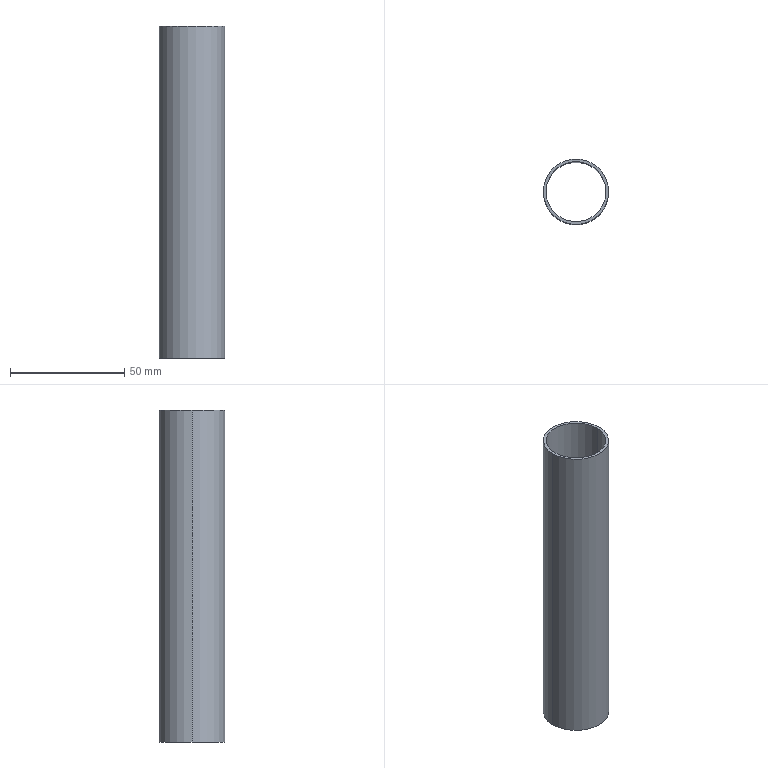Part | STEP file | 28._28.6X145 | 1 solid | 6 faces | box 28.6 x 28.6 x 145 mm | volume 14978 mm3 | cylinder 4 | plane 2 | commonest cylinder face diameters 26.2 x2 28.6 x2
STEP:
#1=CARTESIAN_POINT('',(13.1,0.,0.));
#2=VERTEX_POINT('',#1);
#3=CARTESIAN_POINT('',(-13.1,0.,0.));
#4=VERTEX_POINT('',#3);
#5=CARTESIAN_POINT('',(0.,0.,0.));
#6=DIRECTION('',(0.,0.,-1.));
#7=DIRECTION('',(1.,0.,0.));
#8=AXIS2_PLACEMENT_3D('',#5,#6,#7);
#9=CIRCLE('',#8,13.1);
#10=EDGE_CURVE('',#2,#4,#9,.T.);
#11=ORIENTED_EDGE('',*,*,#10,.T.);
#12=CARTESIAN_POINT('',(-13.1,0.,145.));
#13=VERTEX_POINT('',#12);
#14=CARTESIAN_POINT('',(-13.1,0.,0.));
#15=DIRECTION('',(0.,0.,1.));
#16=VECTOR('',#15,1000.);
#17=LINE('',#14,#16);
#18=EDGE_CURVE('',#4,#13,#17,.T.);
#19=ORIENTED_EDGE('',*,*,#18,.T.);
#20=CARTESIAN_POINT('',(13.1,0.,145.));
#21=VERTEX_POINT('',#20);
#22=CARTESIAN_POINT('',(0.,0.,145.));
#23=DIRECTION('',(0.,0.,-1.));
#24=DIRECTION('',(1.,0.,0.));
#25=AXIS2_PLACEMENT_3D('',#22,#23,#24);
#26=CIRCLE('',#25,13.1);
#27=EDGE_CURVE('',#21,#13,#26,.T.);
#28=ORIENTED_EDGE('',*,*,#27,.F.);
#29=CARTESIAN_POINT('',(13.1,0.,0.));
#30=DIRECTION('',(0.,0.,1.));
#31=VECTOR('',#30,1000.);
#32=LINE('',#29,#31);
#33=EDGE_CURVE('',#2,#21,#32,.T.);
#34=ORIENTED_EDGE('',*,*,#33,.F.);
#35=EDGE_LOOP('',(#11,#19,#28,#34));
#36=FACE_OUTER_BOUND('',#35,.T.);
#37=CARTESIAN_POINT('',(0.,0.,0.));
#38=DIRECTION('',(0.,0.,1.));
#39=DIRECTION('',(1.,0.,0.));
#40=AXIS2_PLACEMENT_3D('',#37,#38,#39);
#41=CYLINDRICAL_SURFACE('',#40,13.1);
#42=ADVANCED_FACE('',(#36),#41,.F.);
#43=CARTESIAN_POINT('',(14.3,0.,0.));
#44=VERTEX_POINT('',#43);
#45=CARTESIAN_POINT('',(-14.3,0.,0.));
#46=VERTEX_POINT('',#45);
#47=CARTESIAN_POINT('',(0.,0.,0.));
#48=DIRECTION('',(0.,0.,1.));
#49=DIRECTION('',(1.,0.,0.));
#50=AXIS2_PLACEMENT_3D('',#47,#48,#49);
#51=CIRCLE('',#50,14.3);
#52=EDGE_CURVE('',#44,#46,#51,.T.);
#53=ORIENTED_EDGE('',*,*,#52,.T.);
#54=CARTESIAN_POINT('',(-14.3,0.,145.));
#55=VERTEX_POINT('',#54);
#56=CARTESIAN_POINT('',(-14.3,0.,0.));
#57=DIRECTION('',(0.,0.,1.));
#58=VECTOR('',#57,1000.);
#59=LINE('',#56,#58);
#60=EDGE_CURVE('',#46,#55,#59,.T.);
#61=ORIENTED_EDGE('',*,*,#60,.T.);
#62=CARTESIAN_POINT('',(14.3,0.,145.));
#63=VERTEX_POINT('',#62);
#64=CARTESIAN_POINT('',(0.,0.,145.));
#65=DIRECTION('',(0.,0.,1.));
#66=DIRECTION('',(1.,0.,0.));
#67=AXIS2_PLACEMENT_3D('',#64,#65,#66);
#68=CIRCLE('',#67,14.3);
#69=EDGE_CURVE('',#63,#55,#68,.T.);
#70=ORIENTED_EDGE('',*,*,#69,.F.);
#71=CARTESIAN_POINT('',(14.3,0.,0.));
#72=DIRECTION('',(0.,0.,1.));
#73=VECTOR('',#72,1000.);
#74=LINE('',#71,#73);
#75=EDGE_CURVE('',#44,#63,#74,.T.);
#76=ORIENTED_EDGE('',*,*,#75,.F.);
#77=EDGE_LOOP('',(#53,#61,#70,#76));
#78=FACE_OUTER_BOUND('',#77,.T.);
#79=CARTESIAN_POINT('',(0.,0.,0.));
#80=DIRECTION('',(0.,0.,1.));
#81=DIRECTION('',(1.,0.,0.));
#82=AXIS2_PLACEMENT_3D('',#79,#80,#81);
#83=CYLINDRICAL_SURFACE('',#82,14.3);
#84=ADVANCED_FACE('',(#78),#83,.T.);
#85=ORIENTED_EDGE('',*,*,#10,.F.);
#86=CARTESIAN_POINT('',(0.,0.,0.));
#87=DIRECTION('',(0.,0.,-1.));
#88=DIRECTION('',(1.,0.,0.));
#89=AXIS2_PLACEMENT_3D('',#86,#87,#88);
#90=CIRCLE('',#89,13.1);
#91=EDGE_CURVE('',#4,#2,#90,.T.);
#92=ORIENTED_EDGE('',*,*,#91,.F.);
#93=EDGE_LOOP('',(#85,#92));
#94=FACE_BOUND('',#93,.T.);
#95=ORIENTED_EDGE('',*,*,#52,.F.);
#96=CARTESIAN_POINT('',(0.,0.,0.));
#97=DIRECTION('',(0.,0.,1.));
#98=DIRECTION('',(1.,0.,0.));
#99=AXIS2_PLACEMENT_3D('',#96,#97,#98);
#100=CIRCLE('',#99,14.3);
#101=EDGE_CURVE('',#46,#44,#100,.T.);
#102=ORIENTED_EDGE('',*,*,#101,.F.);
#103=EDGE_LOOP('',(#95,#102));
#104=FACE_OUTER_BOUND('',#103,.T.);
#105=CARTESIAN_POINT('',(0.,0.,0.));
#106=DIRECTION('',(0.,0.,1.));
#107=DIRECTION('',(1.,0.,0.));
#108=AXIS2_PLACEMENT_3D('',#105,#106,#107);
#109=PLANE('',#108);
#110=ADVANCED_FACE('',(#94,#104),#109,.F.);
#111=ORIENTED_EDGE('',*,*,#27,.T.);
#112=CARTESIAN_POINT('',(0.,0.,145.));
#113=DIRECTION('',(0.,0.,-1.));
#114=DIRECTION('',(1.,0.,0.));
#115=AXIS2_PLACEMENT_3D('',#112,#113,#114);
#116=CIRCLE('',#115,13.1);
#117=EDGE_CURVE('',#13,#21,#116,.T.);
#118=ORIENTED_EDGE('',*,*,#117,.T.);
#119=EDGE_LOOP('',(#111,#118));
#120=FACE_BOUND('',#119,.T.);
#121=ORIENTED_EDGE('',*,*,#69,.T.);
#122=CARTESIAN_POINT('',(0.,0.,145.));
#123=DIRECTION('',(0.,0.,1.));
#124=DIRECTION('',(1.,0.,0.));
#125=AXIS2_PLACEMENT_3D('',#122,#123,#124);
#126=CIRCLE('',#125,14.3);
#127=EDGE_CURVE('',#55,#63,#126,.T.);
#128=ORIENTED_EDGE('',*,*,#127,.T.);
#129=EDGE_LOOP('',(#121,#128));
#130=FACE_OUTER_BOUND('',#129,.T.);
#131=CARTESIAN_POINT('',(0.,0.,145.));
#132=DIRECTION('',(0.,0.,1.));
#133=DIRECTION('',(1.,0.,0.));
#134=AXIS2_PLACEMENT_3D('',#131,#132,#133);
#135=PLANE('',#134);
#136=ADVANCED_FACE('',(#120,#130),#135,.T.);
#137=ORIENTED_EDGE('',*,*,#60,.F.);
#138=ORIENTED_EDGE('',*,*,#101,.T.);
#139=ORIENTED_EDGE('',*,*,#75,.T.);
#140=ORIENTED_EDGE('',*,*,#127,.F.);
#141=EDGE_LOOP('',(#137,#138,#139,#140));
#142=FACE_OUTER_BOUND('',#141,.T.);
#143=CARTESIAN_POINT('',(0.,0.,0.));
#144=DIRECTION('',(0.,0.,1.));
#145=DIRECTION('',(1.,0.,0.));
#146=AXIS2_PLACEMENT_3D('',#143,#144,#145);
#147=CYLINDRICAL_SURFACE('',#146,14.3);
#148=ADVANCED_FACE('',(#142),#147,.T.);
#149=ORIENTED_EDGE('',*,*,#18,.F.);
#150=ORIENTED_EDGE('',*,*,#91,.T.);
#151=ORIENTED_EDGE('',*,*,#33,.T.);
#152=ORIENTED_EDGE('',*,*,#117,.F.);
#153=EDGE_LOOP('',(#149,#150,#151,#152));
#154=FACE_OUTER_BOUND('',#153,.T.);
#155=CARTESIAN_POINT('',(0.,0.,0.));
#156=DIRECTION('',(0.,0.,1.));
#157=DIRECTION('',(1.,0.,0.));
#158=AXIS2_PLACEMENT_3D('',#155,#156,#157);
#159=CYLINDRICAL_SURFACE('',#158,13.1);
#160=ADVANCED_FACE('',(#154),#159,.F.);
#161=CLOSED_SHELL('',(#42,#84,#110,#136,#148,#160));
#162=MANIFOLD_SOLID_BREP('',#161);
#163=CARTESIAN_POINT('',(0.,0.,0.));
#164=DIRECTION('',(0.,0.,1.));
#165=DIRECTION('',(1.,0.,0.));
#166=AXIS2_PLACEMENT_3D('',#163,#164,#165);
#167=(LENGTH_UNIT()NAMED_UNIT(*)SI_UNIT(.MILLI.,.METRE.));
#168=UNCERTAINTY_MEASURE_WITH_UNIT(LENGTH_MEASURE(0.00001),#167,'','');
#169=(NAMED_UNIT(*)PLANE_ANGLE_UNIT()SI_UNIT($,.RADIAN.));
#170=(NAMED_UNIT(*)SI_UNIT($,.STERADIAN.)SOLID_ANGLE_UNIT());
#171=(GEOMETRIC_REPRESENTATION_CONTEXT(3)GLOBAL_UNCERTAINTY_ASSIGNED_CONTEXT((#168))GLOBAL_UNIT_ASSIGNED_CONTEXT((#167,#169,#170))REPRESENTATION_CONTEXT('',''));
#172=ADVANCED_BREP_SHAPE_REPRESENTATION('',(#162,#166),#171);